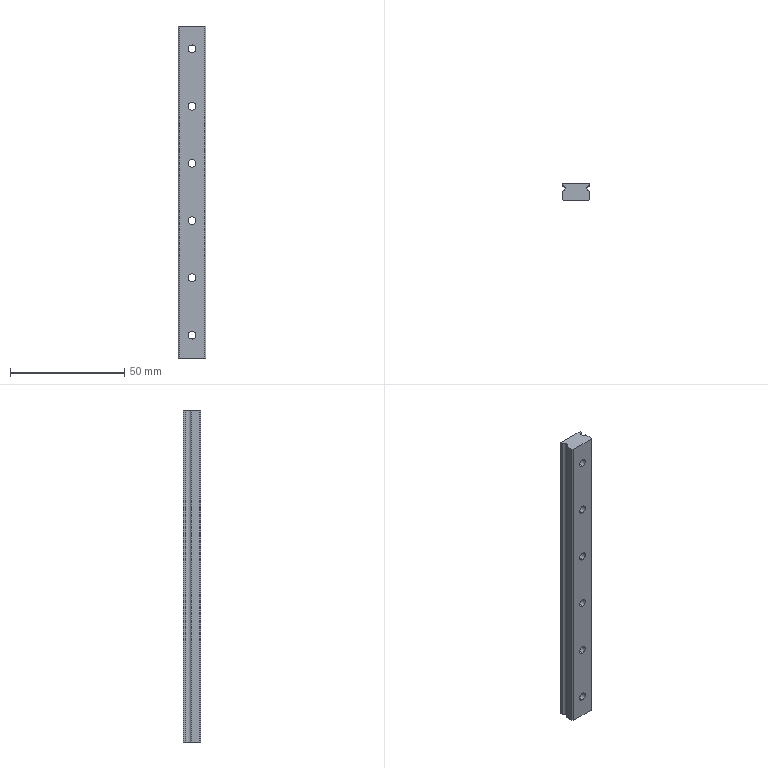Part | NX | features BREP 1 | 1 solid | 43 faces | box 12 x 7.5 x 145 mm | volume 11365 mm3 | cylinder 27 | plane 16 | commonest cylinder face diameters 3.5 x12 6 x12 2.5 x3
STEP:
#1=CARTESIAN_POINT('',(0.,7.5,13.));
#2=VERTEX_POINT('',#1);
#3=CARTESIAN_POINT('',(0.,7.5,7.));
#4=VERTEX_POINT('',#3);
#5=CARTESIAN_POINT('',(0.,7.5,10.));
#6=DIRECTION('',(0.,-1.,0.));
#7=DIRECTION('',(0.,0.,-1.));
#8=AXIS2_PLACEMENT_3D('',#5,#6,#7);
#9=CIRCLE('',#8,3.);
#10=EDGE_CURVE('',#2,#4,#9,.T.);
#11=ORIENTED_EDGE('',*,*,#10,.F.);
#12=CARTESIAN_POINT('',(0.,3.,13.));
#13=VERTEX_POINT('',#12);
#14=CARTESIAN_POINT('',(0.,5.25,13.));
#15=DIRECTION('',(0.,-1.,0.));
#16=VECTOR('',#15,1000.);
#17=LINE('',#14,#16);
#18=EDGE_CURVE('',#2,#13,#17,.T.);
#19=ORIENTED_EDGE('',*,*,#18,.T.);
#20=CARTESIAN_POINT('',(0.,3.,7.));
#21=VERTEX_POINT('',#20);
#22=CARTESIAN_POINT('',(0.,3.,10.));
#23=DIRECTION('',(0.,1.,0.));
#24=DIRECTION('',(0.,0.,-1.));
#25=AXIS2_PLACEMENT_3D('',#22,#23,#24);
#26=CIRCLE('',#25,3.);
#27=EDGE_CURVE('',#21,#13,#26,.T.);
#28=ORIENTED_EDGE('',*,*,#27,.F.);
#29=CARTESIAN_POINT('',(0.,5.25,7.));
#30=DIRECTION('',(0.,-1.,0.));
#31=VECTOR('',#30,1000.);
#32=LINE('',#29,#31);
#33=EDGE_CURVE('',#4,#21,#32,.T.);
#34=ORIENTED_EDGE('',*,*,#33,.F.);
#35=EDGE_LOOP('',(#11,#19,#28,#34));
#36=FACE_BOUND('',#35,.T.);
#37=CARTESIAN_POINT('',(0.,5.25,10.));
#38=DIRECTION('',(0.,-1.,0.));
#39=DIRECTION('',(0.,0.,-1.));
#40=AXIS2_PLACEMENT_3D('',#37,#38,#39);
#41=CYLINDRICAL_SURFACE('',#40,3.);
#42=ADVANCED_FACE('',(#36),#41,.F.);
#43=CARTESIAN_POINT('',(0.,7.5,138.));
#44=VERTEX_POINT('',#43);
#45=CARTESIAN_POINT('',(0.,7.5,132.));
#46=VERTEX_POINT('',#45);
#47=CARTESIAN_POINT('',(0.,7.5,135.));
#48=DIRECTION('',(0.,-1.,0.));
#49=DIRECTION('',(0.,0.,-1.));
#50=AXIS2_PLACEMENT_3D('',#47,#48,#49);
#51=CIRCLE('',#50,3.);
#52=EDGE_CURVE('',#44,#46,#51,.T.);
#53=ORIENTED_EDGE('',*,*,#52,.F.);
#54=CARTESIAN_POINT('',(0.,3.,138.));
#55=VERTEX_POINT('',#54);
#56=CARTESIAN_POINT('',(0.,5.25,138.));
#57=DIRECTION('',(0.,-1.,0.));
#58=VECTOR('',#57,1000.);
#59=LINE('',#56,#58);
#60=EDGE_CURVE('',#44,#55,#59,.T.);
#61=ORIENTED_EDGE('',*,*,#60,.T.);
#62=CARTESIAN_POINT('',(0.,3.,132.));
#63=VERTEX_POINT('',#62);
#64=CARTESIAN_POINT('',(0.,3.,135.));
#65=DIRECTION('',(0.,1.,0.));
#66=DIRECTION('',(0.,0.,-1.));
#67=AXIS2_PLACEMENT_3D('',#64,#65,#66);
#68=CIRCLE('',#67,3.);
#69=EDGE_CURVE('',#63,#55,#68,.T.);
#70=ORIENTED_EDGE('',*,*,#69,.F.);
#71=CARTESIAN_POINT('',(0.,5.25,132.));
#72=DIRECTION('',(0.,-1.,0.));
#73=VECTOR('',#72,1000.);
#74=LINE('',#71,#73);
#75=EDGE_CURVE('',#46,#63,#74,.T.);
#76=ORIENTED_EDGE('',*,*,#75,.F.);
#77=EDGE_LOOP('',(#53,#61,#70,#76));
#78=FACE_BOUND('',#77,.T.);
#79=CARTESIAN_POINT('',(0.,5.25,135.));
#80=DIRECTION('',(0.,-1.,0.));
#81=DIRECTION('',(0.,0.,-1.));
#82=AXIS2_PLACEMENT_3D('',#79,#80,#81);
#83=CYLINDRICAL_SURFACE('',#82,3.);
#84=ADVANCED_FACE('',(#78),#83,.F.);
#85=CARTESIAN_POINT('',(0.,7.5,113.));
#86=VERTEX_POINT('',#85);
#87=CARTESIAN_POINT('',(0.,7.5,107.));
#88=VERTEX_POINT('',#87);
#89=CARTESIAN_POINT('',(0.,7.5,110.));
#90=DIRECTION('',(0.,-1.,0.));
#91=DIRECTION('',(0.,0.,-1.));
#92=AXIS2_PLACEMENT_3D('',#89,#90,#91);
#93=CIRCLE('',#92,3.);
#94=EDGE_CURVE('',#86,#88,#93,.T.);
#95=ORIENTED_EDGE('',*,*,#94,.F.);
#96=CARTESIAN_POINT('',(0.,3.,113.));
#97=VERTEX_POINT('',#96);
#98=CARTESIAN_POINT('',(0.,5.25,113.));
#99=DIRECTION('',(0.,-1.,0.));
#100=VECTOR('',#99,1000.);
#101=LINE('',#98,#100);
#102=EDGE_CURVE('',#86,#97,#101,.T.);
#103=ORIENTED_EDGE('',*,*,#102,.T.);
#104=CARTESIAN_POINT('',(0.,3.,107.));
#105=VERTEX_POINT('',#104);
#106=CARTESIAN_POINT('',(0.,3.,110.));
#107=DIRECTION('',(0.,1.,0.));
#108=DIRECTION('',(0.,0.,-1.));
#109=AXIS2_PLACEMENT_3D('',#106,#107,#108);
#110=CIRCLE('',#109,3.);
#111=EDGE_CURVE('',#105,#97,#110,.T.);
#112=ORIENTED_EDGE('',*,*,#111,.F.);
#113=CARTESIAN_POINT('',(0.,5.25,107.));
#114=DIRECTION('',(0.,-1.,0.));
#115=VECTOR('',#114,1000.);
#116=LINE('',#113,#115);
#117=EDGE_CURVE('',#88,#105,#116,.T.);
#118=ORIENTED_EDGE('',*,*,#117,.F.);
#119=EDGE_LOOP('',(#95,#103,#112,#118));
#120=FACE_BOUND('',#119,.T.);
#121=CARTESIAN_POINT('',(0.,5.25,110.));
#122=DIRECTION('',(0.,-1.,0.));
#123=DIRECTION('',(0.,0.,-1.));
#124=AXIS2_PLACEMENT_3D('',#121,#122,#123);
#125=CYLINDRICAL_SURFACE('',#124,3.);
#126=ADVANCED_FACE('',(#120),#125,.F.);
#127=CARTESIAN_POINT('',(0.,7.5,88.));
#128=VERTEX_POINT('',#127);
#129=CARTESIAN_POINT('',(0.,7.5,82.));
#130=VERTEX_POINT('',#129);
#131=CARTESIAN_POINT('',(0.,7.5,85.));
#132=DIRECTION('',(0.,-1.,0.));
#133=DIRECTION('',(0.,0.,-1.));
#134=AXIS2_PLACEMENT_3D('',#131,#132,#133);
#135=CIRCLE('',#134,3.);
#136=EDGE_CURVE('',#128,#130,#135,.T.);
#137=ORIENTED_EDGE('',*,*,#136,.F.);
#138=CARTESIAN_POINT('',(0.,3.,88.));
#139=VERTEX_POINT('',#138);
#140=CARTESIAN_POINT('',(0.,5.25,88.));
#141=DIRECTION('',(0.,-1.,0.));
#142=VECTOR('',#141,1000.);
#143=LINE('',#140,#142);
#144=EDGE_CURVE('',#128,#139,#143,.T.);
#145=ORIENTED_EDGE('',*,*,#144,.T.);
#146=CARTESIAN_POINT('',(0.,3.,82.));
#147=VERTEX_POINT('',#146);
#148=CARTESIAN_POINT('',(0.,3.,85.));
#149=DIRECTION('',(0.,1.,0.));
#150=DIRECTION('',(0.,0.,-1.));
#151=AXIS2_PLACEMENT_3D('',#148,#149,#150);
#152=CIRCLE('',#151,3.);
#153=EDGE_CURVE('',#147,#139,#152,.T.);
#154=ORIENTED_EDGE('',*,*,#153,.F.);
#155=CARTESIAN_POINT('',(0.,5.25,82.));
#156=DIRECTION('',(0.,-1.,0.));
#157=VECTOR('',#156,1000.);
#158=LINE('',#155,#157);
#159=EDGE_CURVE('',#130,#147,#158,.T.);
#160=ORIENTED_EDGE('',*,*,#159,.F.);
#161=EDGE_LOOP('',(#137,#145,#154,#160));
#162=FACE_BOUND('',#161,.T.);
#163=CARTESIAN_POINT('',(0.,5.25,85.));
#164=DIRECTION('',(0.,-1.,0.));
#165=DIRECTION('',(0.,0.,-1.));
#166=AXIS2_PLACEMENT_3D('',#163,#164,#165);
#167=CYLINDRICAL_SURFACE('',#166,3.);
#168=ADVANCED_FACE('',(#162),#167,.F.);
#169=CARTESIAN_POINT('',(0.,7.5,63.));
#170=VERTEX_POINT('',#169);
#171=CARTESIAN_POINT('',(0.,7.5,57.));
#172=VERTEX_POINT('',#171);
#173=CARTESIAN_POINT('',(0.,7.5,60.));
#174=DIRECTION('',(0.,-1.,0.));
#175=DIRECTION('',(0.,0.,-1.));
#176=AXIS2_PLACEMENT_3D('',#173,#174,#175);
#177=CIRCLE('',#176,3.);
#178=EDGE_CURVE('',#170,#172,#177,.T.);
#179=ORIENTED_EDGE('',*,*,#178,.F.);
#180=CARTESIAN_POINT('',(0.,3.,63.));
#181=VERTEX_POINT('',#180);
#182=CARTESIAN_POINT('',(0.,5.25,63.));
#183=DIRECTION('',(0.,-1.,0.));
#184=VECTOR('',#183,1000.);
#185=LINE('',#182,#184);
#186=EDGE_CURVE('',#170,#181,#185,.T.);
#187=ORIENTED_EDGE('',*,*,#186,.T.);
#188=CARTESIAN_POINT('',(0.,3.,57.));
#189=VERTEX_POINT('',#188);
#190=CARTESIAN_POINT('',(0.,3.,60.));
#191=DIRECTION('',(0.,1.,0.));
#192=DIRECTION('',(0.,0.,-1.));
#193=AXIS2_PLACEMENT_3D('',#190,#191,#192);
#194=CIRCLE('',#193,3.);
#195=EDGE_CURVE('',#189,#181,#194,.T.);
#196=ORIENTED_EDGE('',*,*,#195,.F.);
#197=CARTESIAN_POINT('',(0.,5.25,57.));
#198=DIRECTION('',(0.,-1.,0.));
#199=VECTOR('',#198,1000.);
#200=LINE('',#197,#199);
#201=EDGE_CURVE('',#172,#189,#200,.T.);
#202=ORIENTED_EDGE('',*,*,#201,.F.);
#203=EDGE_LOOP('',(#179,#187,#196,#202));
#204=FACE_BOUND('',#203,.T.);
#205=CARTESIAN_POINT('',(0.,5.25,60.));
#206=DIRECTION('',(0.,-1.,0.));
#207=DIRECTION('',(0.,0.,-1.));
#208=AXIS2_PLACEMENT_3D('',#205,#206,#207);
#209=CYLINDRICAL_SURFACE('',#208,3.);
#210=ADVANCED_FACE('',(#204),#209,.F.);
#211=CARTESIAN_POINT('',(0.,7.5,38.));
#212=VERTEX_POINT('',#211);
#213=CARTESIAN_POINT('',(0.,7.5,32.));
#214=VERTEX_POINT('',#213);
#215=CARTESIAN_POINT('',(0.,7.5,35.));
#216=DIRECTION('',(0.,-1.,0.));
#217=DIRECTION('',(0.,0.,-1.));
#218=AXIS2_PLACEMENT_3D('',#215,#216,#217);
#219=CIRCLE('',#218,3.);
#220=EDGE_CURVE('',#212,#214,#219,.T.);
#221=ORIENTED_EDGE('',*,*,#220,.F.);
#222=CARTESIAN_POINT('',(0.,3.,38.));
#223=VERTEX_POINT('',#222);
#224=CARTESIAN_POINT('',(0.,5.25,38.));
#225=DIRECTION('',(0.,-1.,0.));
#226=VECTOR('',#225,1000.);
#227=LINE('',#224,#226);
#228=EDGE_CURVE('',#212,#223,#227,.T.);
#229=ORIENTED_EDGE('',*,*,#228,.T.);
#230=CARTESIAN_POINT('',(0.,3.,32.));
#231=VERTEX_POINT('',#230);
#232=CARTESIAN_POINT('',(0.,3.,35.));
#233=DIRECTION('',(0.,1.,0.));
#234=DIRECTION('',(0.,0.,-1.));
#235=AXIS2_PLACEMENT_3D('',#232,#233,#234);
#236=CIRCLE('',#235,3.);
#237=EDGE_CURVE('',#231,#223,#236,.T.);
#238=ORIENTED_EDGE('',*,*,#237,.F.);
#239=CARTESIAN_POINT('',(0.,5.25,32.));
#240=DIRECTION('',(0.,-1.,0.));
#241=VECTOR('',#240,1000.);
#242=LINE('',#239,#241);
#243=EDGE_CURVE('',#214,#231,#242,.T.);
#244=ORIENTED_EDGE('',*,*,#243,.F.);
#245=EDGE_LOOP('',(#221,#229,#238,#244));
#246=FACE_BOUND('',#245,.T.);
#247=CARTESIAN_POINT('',(0.,5.25,35.));
#248=DIRECTION('',(0.,-1.,0.));
#249=DIRECTION('',(0.,0.,-1.));
#250=AXIS2_PLACEMENT_3D('',#247,#248,#249);
#251=CYLINDRICAL_SURFACE('',#250,3.);
#252=ADVANCED_FACE('',(#246),#251,.F.);
#253=CARTESIAN_POINT('',(4.75,5.25,145.));
#254=VERTEX_POINT('',#253);
#255=CARTESIAN_POINT('',(6.,6.5,145.));
#256=VERTEX_POINT('',#255);
#257=CARTESIAN_POINT('',(6.,5.25,145.));
#258=DIRECTION('',(0.,0.,-1.));
#259=DIRECTION('',(-1.,0.,0.));
#260=AXIS2_PLACEMENT_3D('',#257,#258,#259);
#261=CIRCLE('',#260,1.25);
#262=EDGE_CURVE('',#254,#256,#261,.T.);
#263=ORIENTED_EDGE('',*,*,#262,.F.);
#264=CARTESIAN_POINT('',(4.75,5.25,0.));
#265=VERTEX_POINT('',#264);
#266=CARTESIAN_POINT('',(4.75,5.25,0.));
#267=DIRECTION('',(0.,0.,-1.));
#268=VECTOR('',#267,1000.);
#269=LINE('',#266,#268);
#270=EDGE_CURVE('',#254,#265,#269,.T.);
#271=ORIENTED_EDGE('',*,*,#270,.T.);
#272=CARTESIAN_POINT('',(6.,6.5,0.));
#273=VERTEX_POINT('',#272);
#274=CARTESIAN_POINT('',(6.,5.25,0.));
#275=DIRECTION('',(0.,0.,-1.));
#276=DIRECTION('',(-1.,0.,0.));
#277=AXIS2_PLACEMENT_3D('',#274,#275,#276);
#278=CIRCLE('',#277,1.25);
#279=EDGE_CURVE('',#265,#273,#278,.T.);
#280=ORIENTED_EDGE('',*,*,#279,.T.);
#281=CARTESIAN_POINT('',(6.,6.5,0.));
#282=DIRECTION('',(0.,0.,-1.));
#283=VECTOR('',#282,1000.);
#284=LINE('',#281,#283);
#285=EDGE_CURVE('',#256,#273,#284,.T.);
#286=ORIENTED_EDGE('',*,*,#285,.F.);
#287=EDGE_LOOP('',(#263,#271,#280,#286));
#288=FACE_BOUND('',#287,.T.);
#289=CARTESIAN_POINT('',(6.,5.25,0.));
#290=DIRECTION('',(0.,0.,-1.));
#291=DIRECTION('',(-1.,0.,0.));
#292=AXIS2_PLACEMENT_3D('',#289,#290,#291);
#293=CYLINDRICAL_SURFACE('',#292,1.25);
#294=ADVANCED_FACE('',(#288),#293,.F.);
#295=CARTESIAN_POINT('',(0.,3.,8.25));
#296=VERTEX_POINT('',#295);
#297=CARTESIAN_POINT('',(0.,3.,11.75));
#298=VERTEX_POINT('',#297);
#299=CARTESIAN_POINT('',(0.,3.,10.));
#300=DIRECTION('',(0.,1.,0.));
#301=DIRECTION('',(0.,0.,-1.));
#302=AXIS2_PLACEMENT_3D('',#299,#300,#301);
#303=CIRCLE('',#302,1.75);
#304=EDGE_CURVE('',#296,#298,#303,.T.);
#305=ORIENTED_EDGE('',*,*,#304,.T.);
#306=CARTESIAN_POINT('',(0.,0.,11.75));
#307=VERTEX_POINT('',#306);
#308=CARTESIAN_POINT('',(0.,1.5,11.75));
#309=DIRECTION('',(0.,-1.,0.));
#310=VECTOR('',#309,1000.);
#311=LINE('',#308,#310);
#312=EDGE_CURVE('',#298,#307,#311,.T.);
#313=ORIENTED_EDGE('',*,*,#312,.T.);
#314=CARTESIAN_POINT('',(0.,0.,8.25));
#315=VERTEX_POINT('',#314);
#316=CARTESIAN_POINT('',(0.,0.,10.));
#317=DIRECTION('',(0.,1.,0.));
#318=DIRECTION('',(0.,0.,-1.));
#319=AXIS2_PLACEMENT_3D('',#316,#317,#318);
#320=CIRCLE('',#319,1.75);
#321=EDGE_CURVE('',#315,#307,#320,.T.);
#322=ORIENTED_EDGE('',*,*,#321,.F.);
#323=CARTESIAN_POINT('',(0.,1.5,8.25));
#324=DIRECTION('',(0.,-1.,0.));
#325=VECTOR('',#324,1000.);
#326=LINE('',#323,#325);
#327=EDGE_CURVE('',#296,#315,#326,.T.);
#328=ORIENTED_EDGE('',*,*,#327,.F.);
#329=EDGE_LOOP('',(#305,#313,#322,#328));
#330=FACE_BOUND('',#329,.T.);
#331=CARTESIAN_POINT('',(0.,1.5,10.));
#332=DIRECTION('',(0.,-1.,0.));
#333=DIRECTION('',(0.,0.,-1.));
#334=AXIS2_PLACEMENT_3D('',#331,#332,#333);
#335=CYLINDRICAL_SURFACE('',#334,1.75);
#336=ADVANCED_FACE('',(#330),#335,.F.);
#337=CARTESIAN_POINT('',(0.,3.,133.25));
#338=VERTEX_POINT('',#337);
#339=CARTESIAN_POINT('',(0.,3.,136.75));
#340=VERTEX_POINT('',#339);
#341=CARTESIAN_POINT('',(0.,3.,135.));
#342=DIRECTION('',(0.,1.,0.));
#343=DIRECTION('',(0.,0.,-1.));
#344=AXIS2_PLACEMENT_3D('',#341,#342,#343);
#345=CIRCLE('',#344,1.75);
#346=EDGE_CURVE('',#338,#340,#345,.T.);
#347=ORIENTED_EDGE('',*,*,#346,.T.);
#348=CARTESIAN_POINT('',(0.,0.,136.75));
#349=VERTEX_POINT('',#348);
#350=CARTESIAN_POINT('',(0.,1.5,136.75));
#351=DIRECTION('',(0.,-1.,0.));
#352=VECTOR('',#351,1000.);
#353=LINE('',#350,#352);
#354=EDGE_CURVE('',#340,#349,#353,.T.);
#355=ORIENTED_EDGE('',*,*,#354,.T.);
#356=CARTESIAN_POINT('',(0.,0.,133.25));
#357=VERTEX_POINT('',#356);
#358=CARTESIAN_POINT('',(0.,0.,135.));
#359=DIRECTION('',(0.,1.,0.));
#360=DIRECTION('',(0.,0.,-1.));
#361=AXIS2_PLACEMENT_3D('',#358,#359,#360);
#362=CIRCLE('',#361,1.75);
#363=EDGE_CURVE('',#357,#349,#362,.T.);
#364=ORIENTED_EDGE('',*,*,#363,.F.);
#365=CARTESIAN_POINT('',(0.,1.5,133.25));
#366=DIRECTION('',(0.,-1.,0.));
#367=VECTOR('',#366,1000.);
#368=LINE('',#365,#367);
#369=EDGE_CURVE('',#338,#357,#368,.T.);
#370=ORIENTED_EDGE('',*,*,#369,.F.);
#371=EDGE_LOOP('',(#347,#355,#364,#370));
#372=FACE_BOUND('',#371,.T.);
#373=CARTESIAN_POINT('',(0.,1.5,135.));
#374=DIRECTION('',(0.,-1.,0.));
#375=DIRECTION('',(0.,0.,-1.));
#376=AXIS2_PLACEMENT_3D('',#373,#374,#375);
#377=CYLINDRICAL_SURFACE('',#376,1.75);
#378=ADVANCED_FACE('',(#372),#377,.F.);
#379=CARTESIAN_POINT('',(0.,3.,108.25));
#380=VERTEX_POINT('',#379);
#381=CARTESIAN_POINT('',(0.,3.,111.75));
#382=VERTEX_POINT('',#381);
#383=CARTESIAN_POINT('',(0.,3.,110.));
#384=DIRECTION('',(0.,1.,0.));
#385=DIRECTION('',(0.,0.,-1.));
#386=AXIS2_PLACEMENT_3D('',#383,#384,#385);
#387=CIRCLE('',#386,1.75);
#388=EDGE_CURVE('',#380,#382,#387,.T.);
#389=ORIENTED_EDGE('',*,*,#388,.T.);
#390=CARTESIAN_POINT('',(0.,0.,111.75));
#391=VERTEX_POINT('',#390);
#392=CARTESIAN_POINT('',(0.,1.5,111.75));
#393=DIRECTION('',(0.,-1.,0.));
#394=VECTOR('',#393,1000.);
#395=LINE('',#392,#394);
#396=EDGE_CURVE('',#382,#391,#395,.T.);
#397=ORIENTED_EDGE('',*,*,#396,.T.);
#398=CARTESIAN_POINT('',(0.,0.,108.25));
#399=VERTEX_POINT('',#398);
#400=CARTESIAN_POINT('',(0.,0.,110.));
#401=DIRECTION('',(0.,1.,0.));
#402=DIRECTION('',(0.,0.,-1.));
#403=AXIS2_PLACEMENT_3D('',#400,#401,#402);
#404=CIRCLE('',#403,1.75);
#405=EDGE_CURVE('',#399,#391,#404,.T.);
#406=ORIENTED_EDGE('',*,*,#405,.F.);
#407=CARTESIAN_POINT('',(0.,1.5,108.25));
#408=DIRECTION('',(0.,-1.,0.));
#409=VECTOR('',#408,1000.);
#410=LINE('',#407,#409);
#411=EDGE_CURVE('',#380,#399,#410,.T.);
#412=ORIENTED_EDGE('',*,*,#411,.F.);
#413=EDGE_LOOP('',(#389,#397,#406,#412));
#414=FACE_BOUND('',#413,.T.);
#415=CARTESIAN_POINT('',(0.,1.5,110.));
#416=DIRECTION('',(0.,-1.,0.));
#417=DIRECTION('',(0.,0.,-1.));
#418=AXIS2_PLACEMENT_3D('',#415,#416,#417);
#419=CYLINDRICAL_SURFACE('',#418,1.75);
#420=ADVANCED_FACE('',(#414),#419,.F.);
#421=CARTESIAN_POINT('',(0.,3.,83.25));
#422=VERTEX_POINT('',#421);
#423=CARTESIAN_POINT('',(0.,3.,86.75));
#424=VERTEX_POINT('',#423);
#425=CARTESIAN_POINT('',(0.,3.,85.));
#426=DIRECTION('',(0.,1.,0.));
#427=DIRECTION('',(0.,0.,-1.));
#428=AXIS2_PLACEMENT_3D('',#425,#426,#427);
#429=CIRCLE('',#428,1.75);
#430=EDGE_CURVE('',#422,#424,#429,.T.);
#431=ORIENTED_EDGE('',*,*,#430,.T.);
#432=CARTESIAN_POINT('',(0.,0.,86.75));
#433=VERTEX_POINT('',#432);
#434=CARTESIAN_POINT('',(0.,1.5,86.75));
#435=DIRECTION('',(0.,-1.,0.));
#436=VECTOR('',#435,1000.);
#437=LINE('',#434,#436);
#438=EDGE_CURVE('',#424,#433,#437,.T.);
#439=ORIENTED_EDGE('',*,*,#438,.T.);
#440=CARTESIAN_POINT('',(0.,0.,83.25));
#441=VERTEX_POINT('',#440);
#442=CARTESIAN_POINT('',(0.,0.,85.));
#443=DIRECTION('',(0.,1.,0.));
#444=DIRECTION('',(0.,0.,-1.));
#445=AXIS2_PLACEMENT_3D('',#442,#443,#444);
#446=CIRCLE('',#445,1.75);
#447=EDGE_CURVE('',#441,#433,#446,.T.);
#448=ORIENTED_EDGE('',*,*,#447,.F.);
#449=CARTESIAN_POINT('',(0.,1.5,83.25));
#450=DIRECTION('',(0.,-1.,0.));
#451=VECTOR('',#450,1000.);
#452=LINE('',#449,#451);
#453=EDGE_CURVE('',#422,#441,#452,.T.);
#454=ORIENTED_EDGE('',*,*,#453,.F.);
#455=EDGE_LOOP('',(#431,#439,#448,#454));
#456=FACE_BOUND('',#455,.T.);
#457=CARTESIAN_POINT('',(0.,1.5,85.));
#458=DIRECTION('',(0.,-1.,0.));
#459=DIRECTION('',(0.,0.,-1.));
#460=AXIS2_PLACEMENT_3D('',#457,#458,#459);
#461=CYLINDRICAL_SURFACE('',#460,1.75);
#462=ADVANCED_FACE('',(#456),#461,.F.);
#463=CARTESIAN_POINT('',(0.,3.,58.25));
#464=VERTEX_POINT('',#463);
#465=CARTESIAN_POINT('',(0.,3.,61.75));
#466=VERTEX_POINT('',#465);
#467=CARTESIAN_POINT('',(0.,3.,60.));
#468=DIRECTION('',(0.,1.,0.));
#469=DIRECTION('',(0.,0.,-1.));
#470=AXIS2_PLACEMENT_3D('',#467,#468,#469);
#471=CIRCLE('',#470,1.75);
#472=EDGE_CURVE('',#464,#466,#471,.T.);
#473=ORIENTED_EDGE('',*,*,#472,.T.);
#474=CARTESIAN_POINT('',(0.,0.,61.75));
#475=VERTEX_POINT('',#474);
#476=CARTESIAN_POINT('',(0.,1.5,61.75));
#477=DIRECTION('',(0.,-1.,0.));
#478=VECTOR('',#477,1000.);
#479=LINE('',#476,#478);
#480=EDGE_CURVE('',#466,#475,#479,.T.);
#481=ORIENTED_EDGE('',*,*,#480,.T.);
#482=CARTESIAN_POINT('',(0.,0.,58.25));
#483=VERTEX_POINT('',#482);
#484=CARTESIAN_POINT('',(0.,0.,60.));
#485=DIRECTION('',(0.,1.,0.));
#486=DIRECTION('',(0.,0.,-1.));
#487=AXIS2_PLACEMENT_3D('',#484,#485,#486);
#488=CIRCLE('',#487,1.75);
#489=EDGE_CURVE('',#483,#475,#488,.T.);
#490=ORIENTED_EDGE('',*,*,#489,.F.);
#491=CARTESIAN_POINT('',(0.,1.5,58.25));
#492=DIRECTION('',(0.,-1.,0.));
#493=VECTOR('',#492,1000.);
#494=LINE('',#491,#493);
#495=EDGE_CURVE('',#464,#483,#494,.T.);
#496=ORIENTED_EDGE('',*,*,#495,.F.);
#497=EDGE_LOOP('',(#473,#481,#490,#496));
#498=FACE_BOUND('',#497,.T.);
#499=CARTESIAN_POINT('',(0.,1.5,60.));
#500=DIRECTION('',(0.,-1.,0.));
#501=DIRECTION('',(0.,0.,-1.));
#502=AXIS2_PLACEMENT_3D('',#499,#500,#501);
#503=CYLINDRICAL_SURFACE('',#502,1.75);
#504=ADVANCED_FACE('',(#498),#503,.F.);
#505=CARTESIAN_POINT('',(0.,3.,33.25));
#506=VERTEX_POINT('',#505);
#507=CARTESIAN_POINT('',(0.,3.,36.75));
#508=VERTEX_POINT('',#507);
#509=CARTESIAN_POINT('',(0.,3.,35.));
#510=DIRECTION('',(0.,1.,0.));
#511=DIRECTION('',(0.,0.,-1.));
#512=AXIS2_PLACEMENT_3D('',#509,#510,#511);
#513=CIRCLE('',#512,1.75);
#514=EDGE_CURVE('',#506,#508,#513,.T.);
#515=ORIENTED_EDGE('',*,*,#514,.T.);
#516=CARTESIAN_POINT('',(0.,0.,36.75));
#517=VERTEX_POINT('',#516);
#518=CARTESIAN_POINT('',(0.,1.5,36.75));
#519=DIRECTION('',(0.,-1.,0.));
#520=VECTOR('',#519,1000.);
#521=LINE('',#518,#520);
#522=EDGE_CURVE('',#508,#517,#521,.T.);
#523=ORIENTED_EDGE('',*,*,#522,.T.);
#524=CARTESIAN_POINT('',(0.,0.,33.25));
#525=VERTEX_POINT('',#524);
#526=CARTESIAN_POINT('',(0.,0.,35.));
#527=DIRECTION('',(0.,1.,0.));
#528=DIRECTION('',(0.,0.,-1.));
#529=AXIS2_PLACEMENT_3D('',#526,#527,#528);
#530=CIRCLE('',#529,1.75);
#531=EDGE_CURVE('',#525,#517,#530,.T.);
#532=ORIENTED_EDGE('',*,*,#531,.F.);
#533=CARTESIAN_POINT('',(0.,1.5,33.25));
#534=DIRECTION('',(0.,-1.,0.));
#535=VECTOR('',#534,1000.);
#536=LINE('',#533,#535);
#537=EDGE_CURVE('',#506,#525,#536,.T.);
#538=ORIENTED_EDGE('',*,*,#537,.F.);
#539=EDGE_LOOP('',(#515,#523,#532,#538));
#540=FACE_BOUND('',#539,.T.);
#541=CARTESIAN_POINT('',(0.,1.5,35.));
#542=DIRECTION('',(0.,-1.,0.));
#543=DIRECTION('',(0.,0.,-1.));
#544=AXIS2_PLACEMENT_3D('',#541,#542,#543);
#545=CYLINDRICAL_SURFACE('',#544,1.75);
#546=ADVANCED_FACE('',(#540),#545,.F.);
#547=CARTESIAN_POINT('',(6.,7.5,0.));
#548=VERTEX_POINT('',#547);
#549=CARTESIAN_POINT('',(-6.,7.5,0.));
#550=VERTEX_POINT('',#549);
#551=CARTESIAN_POINT('',(-6.,7.5,0.));
#552=DIRECTION('',(-1.,0.,0.));
#553=VECTOR('',#552,1000.);
#554=LINE('',#551,#553);
#555=EDGE_CURVE('',#548,#550,#554,.T.);
#556=ORIENTED_EDGE('',*,*,#555,.T.);
#557=CARTESIAN_POINT('',(-6.,7.5,145.));
#558=VERTEX_POINT('',#557);
#559=CARTESIAN_POINT('',(-6.,7.5,0.));
#560=DIRECTION('',(0.,0.,1.));
#561=VECTOR('',#560,1000.);
#562=LINE('',#559,#561);
#563=EDGE_CURVE('',#550,#558,#562,.T.);
#564=ORIENTED_EDGE('',*,*,#563,.T.);
#565=CARTESIAN_POINT('',(6.,7.5,145.));
#566=VERTEX_POINT('',#565);
#567=CARTESIAN_POINT('',(-6.,7.5,145.));
#568=DIRECTION('',(1.,0.,0.));
#569=VECTOR('',#568,1000.);
#570=LINE('',#567,#569);
#571=EDGE_CURVE('',#558,#566,#570,.T.);
#572=ORIENTED_EDGE('',*,*,#571,.T.);
#573=CARTESIAN_POINT('',(6.,7.5,0.));
#574=DIRECTION('',(0.,0.,-1.));
#575=VECTOR('',#574,1000.);
#576=LINE('',#573,#575);
#577=EDGE_CURVE('',#566,#548,#576,.T.);
#578=ORIENTED_EDGE('',*,*,#577,.T.);
#579=EDGE_LOOP('',(#556,#564,#572,#578));
#580=FACE_BOUND('',#579,.T.);
#581=CARTESIAN_POINT('',(0.,7.5,10.));
#582=DIRECTION('',(0.,-1.,0.));
#583=DIRECTION('',(0.,0.,-1.));
#584=AXIS2_PLACEMENT_3D('',#581,#582,#583);
#585=CIRCLE('',#584,3.);
#586=EDGE_CURVE('',#4,#2,#585,.T.);
#587=ORIENTED_EDGE('',*,*,#586,.T.);
#588=ORIENTED_EDGE('',*,*,#10,.T.);
#589=EDGE_LOOP('',(#587,#588));
#590=FACE_BOUND('',#589,.T.);
#591=CARTESIAN_POINT('',(0.,7.5,135.));
#592=DIRECTION('',(0.,-1.,0.));
#593=DIRECTION('',(0.,0.,-1.));
#594=AXIS2_PLACEMENT_3D('',#591,#592,#593);
#595=CIRCLE('',#594,3.);
#596=EDGE_CURVE('',#46,#44,#595,.T.);
#597=ORIENTED_EDGE('',*,*,#596,.T.);
#598=ORIENTED_EDGE('',*,*,#52,.T.);
#599=EDGE_LOOP('',(#597,#598));
#600=FACE_BOUND('',#599,.T.);
#601=CARTESIAN_POINT('',(0.,7.5,110.));
#602=DIRECTION('',(0.,-1.,0.));
#603=DIRECTION('',(0.,0.,-1.));
#604=AXIS2_PLACEMENT_3D('',#601,#602,#603);
#605=CIRCLE('',#604,3.);
#606=EDGE_CURVE('',#88,#86,#605,.T.);
#607=ORIENTED_EDGE('',*,*,#606,.T.);
#608=ORIENTED_EDGE('',*,*,#94,.T.);
#609=EDGE_LOOP('',(#607,#608));
#610=FACE_BOUND('',#609,.T.);
#611=CARTESIAN_POINT('',(0.,7.5,85.));
#612=DIRECTION('',(0.,-1.,0.));
#613=DIRECTION('',(0.,0.,-1.));
#614=AXIS2_PLACEMENT_3D('',#611,#612,#613);
#615=CIRCLE('',#614,3.);
#616=EDGE_CURVE('',#130,#128,#615,.T.);
#617=ORIENTED_EDGE('',*,*,#616,.T.);
#618=ORIENTED_EDGE('',*,*,#136,.T.);
#619=EDGE_LOOP('',(#617,#618));
#620=FACE_BOUND('',#619,.T.);
#621=CARTESIAN_POINT('',(0.,7.5,60.));
#622=DIRECTION('',(0.,-1.,0.));
#623=DIRECTION('',(0.,0.,-1.));
#624=AXIS2_PLACEMENT_3D('',#621,#622,#623);
#625=CIRCLE('',#624,3.);
#626=EDGE_CURVE('',#172,#170,#625,.T.);
#627=ORIENTED_EDGE('',*,*,#626,.T.);
#628=ORIENTED_EDGE('',*,*,#178,.T.);
#629=EDGE_LOOP('',(#627,#628));
#630=FACE_BOUND('',#629,.T.);
#631=CARTESIAN_POINT('',(0.,7.5,35.));
#632=DIRECTION('',(0.,-1.,0.));
#633=DIRECTION('',(0.,0.,-1.));
#634=AXIS2_PLACEMENT_3D('',#631,#632,#633);
#635=CIRCLE('',#634,3.);
#636=EDGE_CURVE('',#214,#212,#635,.T.);
#637=ORIENTED_EDGE('',*,*,#636,.T.);
#638=ORIENTED_EDGE('',*,*,#220,.T.);
#639=EDGE_LOOP('',(#637,#638));
#640=FACE_BOUND('',#639,.T.);
#641=CARTESIAN_POINT('',(-6.,7.5,0.));
#642=DIRECTION('',(0.,1.,0.));
#643=DIRECTION('',(1.,0.,0.));
#644=AXIS2_PLACEMENT_3D('',#641,#642,#643);
#645=PLANE('',#644);
#646=ADVANCED_FACE('',(#580,#590,#600,#610,#620,#630,#640),#645,.T.);
#647=CARTESIAN_POINT('',(-6.,6.5,0.));
#648=VERTEX_POINT('',#647);
#649=CARTESIAN_POINT('',(-6.,6.5,0.));
#650=DIRECTION('',(0.,-1.,0.));
#651=VECTOR('',#650,1000.);
#652=LINE('',#649,#651);
#653=EDGE_CURVE('',#550,#648,#652,.T.);
#654=ORIENTED_EDGE('',*,*,#653,.T.);
#655=CARTESIAN_POINT('',(-6.,6.5,145.));
#656=VERTEX_POINT('',#655);
#657=CARTESIAN_POINT('',(-6.,6.5,0.));
#658=DIRECTION('',(0.,0.,1.));
#659=VECTOR('',#658,1000.);
#660=LINE('',#657,#659);
#661=EDGE_CURVE('',#648,#656,#660,.T.);
#662=ORIENTED_EDGE('',*,*,#661,.T.);
#663=CARTESIAN_POINT('',(-6.,6.5,145.));
#664=DIRECTION('',(0.,1.,0.));
#665=VECTOR('',#664,1000.);
#666=LINE('',#663,#665);
#667=EDGE_CURVE('',#656,#558,#666,.T.);
#668=ORIENTED_EDGE('',*,*,#667,.T.);
#669=ORIENTED_EDGE('',*,*,#563,.F.);
#670=EDGE_LOOP('',(#654,#662,#668,#669));
#671=FACE_BOUND('',#670,.T.);
#672=CARTESIAN_POINT('',(-6.,6.5,0.));
#673=DIRECTION('',(-1.,0.,0.));
#674=DIRECTION('',(0.,0.,1.));
#675=AXIS2_PLACEMENT_3D('',#672,#673,#674);
#676=PLANE('',#675);
#677=ADVANCED_FACE('',(#671),#676,.T.);
#678=ORIENTED_EDGE('',*,*,#555,.F.);
#679=CARTESIAN_POINT('',(6.,0.,0.));
#680=DIRECTION('',(0.,1.,0.));
#681=VECTOR('',#680,1000.);
#682=LINE('',#679,#681);
#683=EDGE_CURVE('',#273,#548,#682,.T.);
#684=ORIENTED_EDGE('',*,*,#683,.F.);
#685=ORIENTED_EDGE('',*,*,#279,.F.);
#686=CARTESIAN_POINT('',(6.,4.,0.));
#687=VERTEX_POINT('',#686);
#688=CARTESIAN_POINT('',(6.,5.25,0.));
#689=DIRECTION('',(0.,0.,-1.));
#690=DIRECTION('',(-1.,0.,0.));
#691=AXIS2_PLACEMENT_3D('',#688,#689,#690);
#692=CIRCLE('',#691,1.25);
#693=EDGE_CURVE('',#687,#265,#692,.T.);
#694=ORIENTED_EDGE('',*,*,#693,.F.);
#695=CARTESIAN_POINT('',(6.,0.5,0.));
#696=VERTEX_POINT('',#695);
#697=CARTESIAN_POINT('',(6.,0.,0.));
#698=DIRECTION('',(0.,1.,0.));
#699=VECTOR('',#698,1000.);
#700=LINE('',#697,#699);
#701=EDGE_CURVE('',#696,#687,#700,.T.);
#702=ORIENTED_EDGE('',*,*,#701,.F.);
#703=CARTESIAN_POINT('',(5.5,0.,0.));
#704=VERTEX_POINT('',#703);
#705=CARTESIAN_POINT('',(6.,0.5,0.));
#706=DIRECTION('',(0.7071,0.7071,0.));
#707=VECTOR('',#706,1000.);
#708=LINE('',#705,#707);
#709=EDGE_CURVE('',#704,#696,#708,.T.);
#710=ORIENTED_EDGE('',*,*,#709,.F.);
#711=CARTESIAN_POINT('',(-5.5,0.,0.));
#712=VERTEX_POINT('',#711);
#713=CARTESIAN_POINT('',(0.,0.,0.));
#714=DIRECTION('',(1.,0.,0.));
#715=VECTOR('',#714,1000.);
#716=LINE('',#713,#715);
#717=EDGE_CURVE('',#712,#704,#716,.T.);
#718=ORIENTED_EDGE('',*,*,#717,.F.);
#719=CARTESIAN_POINT('',(-6.,0.5,0.));
#720=VERTEX_POINT('',#719);
#721=CARTESIAN_POINT('',(-5.5,0.,0.));
#722=DIRECTION('',(0.7071,-0.7071,0.));
#723=VECTOR('',#722,1000.);
#724=LINE('',#721,#723);
#725=EDGE_CURVE('',#720,#712,#724,.T.);
#726=ORIENTED_EDGE('',*,*,#725,.F.);
#727=CARTESIAN_POINT('',(-6.,4.,0.));
#728=VERTEX_POINT('',#727);
#729=CARTESIAN_POINT('',(-6.,0.,0.));
#730=DIRECTION('',(0.,-1.,0.));
#731=VECTOR('',#730,1000.);
#732=LINE('',#729,#731);
#733=EDGE_CURVE('',#728,#720,#732,.T.);
#734=ORIENTED_EDGE('',*,*,#733,.F.);
#735=CARTESIAN_POINT('',(-6.,5.25,0.));
#736=DIRECTION('',(0.,0.,-1.));
#737=DIRECTION('',(-1.,0.,0.));
#738=AXIS2_PLACEMENT_3D('',#735,#736,#737);
#739=CIRCLE('',#738,1.25);
#740=EDGE_CURVE('',#648,#728,#739,.T.);
#741=ORIENTED_EDGE('',*,*,#740,.F.);
#742=ORIENTED_EDGE('',*,*,#653,.F.);
#743=EDGE_LOOP('',(#678,#684,#685,#694,#702,#710,#718,#726,#734,#741,#742));
#744=FACE_BOUND('',#743,.T.);
#745=CARTESIAN_POINT('',(0.,0.,0.));
#746=DIRECTION('',(0.,0.,1.));
#747=DIRECTION('',(1.,0.,0.));
#748=AXIS2_PLACEMENT_3D('',#745,#746,#747);
#749=PLANE('',#748);
#750=ADVANCED_FACE('',(#744),#749,.F.);
#751=ORIENTED_EDGE('',*,*,#683,.T.);
#752=ORIENTED_EDGE('',*,*,#577,.F.);
#753=CARTESIAN_POINT('',(6.,7.5,145.));
#754=DIRECTION('',(0.,-1.,0.));
#755=VECTOR('',#754,1000.);
#756=LINE('',#753,#755);
#757=EDGE_CURVE('',#566,#256,#756,.T.);
#758=ORIENTED_EDGE('',*,*,#757,.T.);
#759=ORIENTED_EDGE('',*,*,#285,.T.);
#760=EDGE_LOOP('',(#751,#752,#758,#759));
#761=FACE_BOUND('',#760,.T.);
#762=CARTESIAN_POINT('',(6.,7.5,0.));
#763=DIRECTION('',(1.,0.,0.));
#764=DIRECTION('',(0.,1.,0.));
#765=AXIS2_PLACEMENT_3D('',#762,#763,#764);
#766=PLANE('',#765);
#767=ADVANCED_FACE('',(#761),#766,.T.);
#768=CARTESIAN_POINT('',(6.,4.,145.));
#769=VERTEX_POINT('',#768);
#770=CARTESIAN_POINT('',(6.,5.25,145.));
#771=DIRECTION('',(0.,0.,-1.));
#772=DIRECTION('',(-1.,0.,0.));
#773=AXIS2_PLACEMENT_3D('',#770,#771,#772);
#774=CIRCLE('',#773,1.25);
#775=EDGE_CURVE('',#769,#254,#774,.T.);
#776=ORIENTED_EDGE('',*,*,#775,.T.);
#777=ORIENTED_EDGE('',*,*,#262,.T.);
#778=ORIENTED_EDGE('',*,*,#757,.F.);
#779=ORIENTED_EDGE('',*,*,#571,.F.);
#780=ORIENTED_EDGE('',*,*,#667,.F.);
#781=CARTESIAN_POINT('',(-6.,4.,145.));
#782=VERTEX_POINT('',#781);
#783=CARTESIAN_POINT('',(-6.,5.25,145.));
#784=DIRECTION('',(0.,0.,-1.));
#785=DIRECTION('',(-1.,0.,0.));
#786=AXIS2_PLACEMENT_3D('',#783,#784,#785);
#787=CIRCLE('',#786,1.25);
#788=EDGE_CURVE('',#656,#782,#787,.T.);
#789=ORIENTED_EDGE('',*,*,#788,.T.);
#790=CARTESIAN_POINT('',(-6.,0.5,145.));
#791=VERTEX_POINT('',#790);
#792=CARTESIAN_POINT('',(-6.,0.,145.));
#793=DIRECTION('',(0.,-1.,0.));
#794=VECTOR('',#793,1000.);
#795=LINE('',#792,#794);
#796=EDGE_CURVE('',#782,#791,#795,.T.);
#797=ORIENTED_EDGE('',*,*,#796,.T.);
#798=CARTESIAN_POINT('',(-5.5,0.,145.));
#799=VERTEX_POINT('',#798);
#800=CARTESIAN_POINT('',(-5.5,0.,145.));
#801=DIRECTION('',(-0.7071,0.7071,0.));
#802=VECTOR('',#801,1000.);
#803=LINE('',#800,#802);
#804=EDGE_CURVE('',#799,#791,#803,.T.);
#805=ORIENTED_EDGE('',*,*,#804,.F.);
#806=CARTESIAN_POINT('',(5.5,0.,145.));
#807=VERTEX_POINT('',#806);
#808=CARTESIAN_POINT('',(0.,0.,145.));
#809=DIRECTION('',(1.,0.,0.));
#810=VECTOR('',#809,1000.);
#811=LINE('',#808,#810);
#812=EDGE_CURVE('',#799,#807,#811,.T.);
#813=ORIENTED_EDGE('',*,*,#812,.T.);
#814=CARTESIAN_POINT('',(6.,0.5,145.));
#815=VERTEX_POINT('',#814);
#816=CARTESIAN_POINT('',(6.,0.5,145.));
#817=DIRECTION('',(-0.7071,-0.7071,0.));
#818=VECTOR('',#817,1000.);
#819=LINE('',#816,#818);
#820=EDGE_CURVE('',#815,#807,#819,.T.);
#821=ORIENTED_EDGE('',*,*,#820,.F.);
#822=CARTESIAN_POINT('',(6.,0.,145.));
#823=DIRECTION('',(0.,1.,0.));
#824=VECTOR('',#823,1000.);
#825=LINE('',#822,#824);
#826=EDGE_CURVE('',#815,#769,#825,.T.);
#827=ORIENTED_EDGE('',*,*,#826,.T.);
#828=EDGE_LOOP('',(#776,#777,#778,#779,#780,#789,#797,#805,#813,#821,#827));
#829=FACE_BOUND('',#828,.T.);
#830=CARTESIAN_POINT('',(0.,0.,145.));
#831=DIRECTION('',(0.,0.,1.));
#832=DIRECTION('',(1.,0.,0.));
#833=AXIS2_PLACEMENT_3D('',#830,#831,#832);
#834=PLANE('',#833);
#835=ADVANCED_FACE('',(#829),#834,.T.);
#836=ORIENTED_EDGE('',*,*,#18,.F.);
#837=ORIENTED_EDGE('',*,*,#586,.F.);
#838=ORIENTED_EDGE('',*,*,#33,.T.);
#839=CARTESIAN_POINT('',(0.,3.,10.));
#840=DIRECTION('',(0.,1.,0.));
#841=DIRECTION('',(0.,0.,-1.));
#842=AXIS2_PLACEMENT_3D('',#839,#840,#841);
#843=CIRCLE('',#842,3.);
#844=EDGE_CURVE('',#13,#21,#843,.T.);
#845=ORIENTED_EDGE('',*,*,#844,.F.);
#846=EDGE_LOOP('',(#836,#837,#838,#845));
#847=FACE_BOUND('',#846,.T.);
#848=CARTESIAN_POINT('',(0.,5.25,10.));
#849=DIRECTION('',(0.,-1.,0.));
#850=DIRECTION('',(0.,0.,-1.));
#851=AXIS2_PLACEMENT_3D('',#848,#849,#850);
#852=CYLINDRICAL_SURFACE('',#851,3.);
#853=ADVANCED_FACE('',(#847),#852,.F.);
#854=ORIENTED_EDGE('',*,*,#60,.F.);
#855=ORIENTED_EDGE('',*,*,#596,.F.);
#856=ORIENTED_EDGE('',*,*,#75,.T.);
#857=CARTESIAN_POINT('',(0.,3.,135.));
#858=DIRECTION('',(0.,1.,0.));
#859=DIRECTION('',(0.,0.,-1.));
#860=AXIS2_PLACEMENT_3D('',#857,#858,#859);
#861=CIRCLE('',#860,3.);
#862=EDGE_CURVE('',#55,#63,#861,.T.);
#863=ORIENTED_EDGE('',*,*,#862,.F.);
#864=EDGE_LOOP('',(#854,#855,#856,#863));
#865=FACE_BOUND('',#864,.T.);
#866=CARTESIAN_POINT('',(0.,5.25,135.));
#867=DIRECTION('',(0.,-1.,0.));
#868=DIRECTION('',(0.,0.,-1.));
#869=AXIS2_PLACEMENT_3D('',#866,#867,#868);
#870=CYLINDRICAL_SURFACE('',#869,3.);
#871=ADVANCED_FACE('',(#865),#870,.F.);
#872=ORIENTED_EDGE('',*,*,#102,.F.);
#873=ORIENTED_EDGE('',*,*,#606,.F.);
#874=ORIENTED_EDGE('',*,*,#117,.T.);
#875=CARTESIAN_POINT('',(0.,3.,110.));
#876=DIRECTION('',(0.,1.,0.));
#877=DIRECTION('',(0.,0.,-1.));
#878=AXIS2_PLACEMENT_3D('',#875,#876,#877);
#879=CIRCLE('',#878,3.);
#880=EDGE_CURVE('',#97,#105,#879,.T.);
#881=ORIENTED_EDGE('',*,*,#880,.F.);
#882=EDGE_LOOP('',(#872,#873,#874,#881));
#883=FACE_BOUND('',#882,.T.);
#884=CARTESIAN_POINT('',(0.,5.25,110.));
#885=DIRECTION('',(0.,-1.,0.));
#886=DIRECTION('',(0.,0.,-1.));
#887=AXIS2_PLACEMENT_3D('',#884,#885,#886);
#888=CYLINDRICAL_SURFACE('',#887,3.);
#889=ADVANCED_FACE('',(#883),#888,.F.);
#890=ORIENTED_EDGE('',*,*,#144,.F.);
#891=ORIENTED_EDGE('',*,*,#616,.F.);
#892=ORIENTED_EDGE('',*,*,#159,.T.);
#893=CARTESIAN_POINT('',(0.,3.,85.));
#894=DIRECTION('',(0.,1.,0.));
#895=DIRECTION('',(0.,0.,-1.));
#896=AXIS2_PLACEMENT_3D('',#893,#894,#895);
#897=CIRCLE('',#896,3.);
#898=EDGE_CURVE('',#139,#147,#897,.T.);
#899=ORIENTED_EDGE('',*,*,#898,.F.);
#900=EDGE_LOOP('',(#890,#891,#892,#899));
#901=FACE_BOUND('',#900,.T.);
#902=CARTESIAN_POINT('',(0.,5.25,85.));
#903=DIRECTION('',(0.,-1.,0.));
#904=DIRECTION('',(0.,0.,-1.));
#905=AXIS2_PLACEMENT_3D('',#902,#903,#904);
#906=CYLINDRICAL_SURFACE('',#905,3.);
#907=ADVANCED_FACE('',(#901),#906,.F.);
#908=ORIENTED_EDGE('',*,*,#186,.F.);
#909=ORIENTED_EDGE('',*,*,#626,.F.);
#910=ORIENTED_EDGE('',*,*,#201,.T.);
#911=CARTESIAN_POINT('',(0.,3.,60.));
#912=DIRECTION('',(0.,1.,0.));
#913=DIRECTION('',(0.,0.,-1.));
#914=AXIS2_PLACEMENT_3D('',#911,#912,#913);
#915=CIRCLE('',#914,3.);
#916=EDGE_CURVE('',#181,#189,#915,.T.);
#917=ORIENTED_EDGE('',*,*,#916,.F.);
#918=EDGE_LOOP('',(#908,#909,#910,#917));
#919=FACE_BOUND('',#918,.T.);
#920=CARTESIAN_POINT('',(0.,5.25,60.));
#921=DIRECTION('',(0.,-1.,0.));
#922=DIRECTION('',(0.,0.,-1.));
#923=AXIS2_PLACEMENT_3D('',#920,#921,#922);
#924=CYLINDRICAL_SURFACE('',#923,3.);
#925=ADVANCED_FACE('',(#919),#924,.F.);
#926=ORIENTED_EDGE('',*,*,#228,.F.);
#927=ORIENTED_EDGE('',*,*,#636,.F.);
#928=ORIENTED_EDGE('',*,*,#243,.T.);
#929=CARTESIAN_POINT('',(0.,3.,35.));
#930=DIRECTION('',(0.,1.,0.));
#931=DIRECTION('',(0.,0.,-1.));
#932=AXIS2_PLACEMENT_3D('',#929,#930,#931);
#933=CIRCLE('',#932,3.);
#934=EDGE_CURVE('',#223,#231,#933,.T.);
#935=ORIENTED_EDGE('',*,*,#934,.F.);
#936=EDGE_LOOP('',(#926,#927,#928,#935));
#937=FACE_BOUND('',#936,.T.);
#938=CARTESIAN_POINT('',(0.,5.25,35.));
#939=DIRECTION('',(0.,-1.,0.));
#940=DIRECTION('',(0.,0.,-1.));
#941=AXIS2_PLACEMENT_3D('',#938,#939,#940);
#942=CYLINDRICAL_SURFACE('',#941,3.);
#943=ADVANCED_FACE('',(#937),#942,.F.);
#944=ORIENTED_EDGE('',*,*,#661,.F.);
#945=ORIENTED_EDGE('',*,*,#740,.T.);
#946=CARTESIAN_POINT('',(-6.,4.,0.));
#947=DIRECTION('',(0.,0.,-1.));
#948=VECTOR('',#947,1000.);
#949=LINE('',#946,#948);
#950=EDGE_CURVE('',#782,#728,#949,.T.);
#951=ORIENTED_EDGE('',*,*,#950,.F.);
#952=ORIENTED_EDGE('',*,*,#788,.F.);
#953=EDGE_LOOP('',(#944,#945,#951,#952));
#954=FACE_BOUND('',#953,.T.);
#955=CARTESIAN_POINT('',(-6.,5.25,0.));
#956=DIRECTION('',(0.,0.,-1.));
#957=DIRECTION('',(-1.,0.,0.));
#958=AXIS2_PLACEMENT_3D('',#955,#956,#957);
#959=CYLINDRICAL_SURFACE('',#958,1.25);
#960=ADVANCED_FACE('',(#954),#959,.F.);
#961=ORIENTED_EDGE('',*,*,#270,.F.);
#962=ORIENTED_EDGE('',*,*,#775,.F.);
#963=CARTESIAN_POINT('',(6.,4.,0.));
#964=DIRECTION('',(0.,0.,1.));
#965=VECTOR('',#964,1000.);
#966=LINE('',#963,#965);
#967=EDGE_CURVE('',#687,#769,#966,.T.);
#968=ORIENTED_EDGE('',*,*,#967,.F.);
#969=ORIENTED_EDGE('',*,*,#693,.T.);
#970=EDGE_LOOP('',(#961,#962,#968,#969));
#971=FACE_BOUND('',#970,.T.);
#972=CARTESIAN_POINT('',(6.,5.25,0.));
#973=DIRECTION('',(0.,0.,-1.));
#974=DIRECTION('',(-1.,0.,0.));
#975=AXIS2_PLACEMENT_3D('',#972,#973,#974);
#976=CYLINDRICAL_SURFACE('',#975,1.25);
#977=ADVANCED_FACE('',(#971),#976,.F.);
#978=ORIENTED_EDGE('',*,*,#701,.T.);
#979=ORIENTED_EDGE('',*,*,#967,.T.);
#980=ORIENTED_EDGE('',*,*,#826,.F.);
#981=CARTESIAN_POINT('',(6.,0.5,0.));
#982=DIRECTION('',(0.,0.,-1.));
#983=VECTOR('',#982,1000.);
#984=LINE('',#981,#983);
#985=EDGE_CURVE('',#815,#696,#984,.T.);
#986=ORIENTED_EDGE('',*,*,#985,.T.);
#987=EDGE_LOOP('',(#978,#979,#980,#986));
#988=FACE_BOUND('',#987,.T.);
#989=CARTESIAN_POINT('',(6.,4.,0.));
#990=DIRECTION('',(1.,0.,0.));
#991=DIRECTION('',(0.,1.,0.));
#992=AXIS2_PLACEMENT_3D('',#989,#990,#991);
#993=PLANE('',#992);
#994=ADVANCED_FACE('',(#988),#993,.T.);
#995=ORIENTED_EDGE('',*,*,#717,.T.);
#996=CARTESIAN_POINT('',(5.5,0.,0.));
#997=DIRECTION('',(0.,0.,1.));
#998=VECTOR('',#997,1000.);
#999=LINE('',#996,#998);
#1000=EDGE_CURVE('',#704,#807,#999,.T.);
#1001=ORIENTED_EDGE('',*,*,#1000,.T.);
#1002=ORIENTED_EDGE('',*,*,#812,.F.);
#1003=CARTESIAN_POINT('',(-5.5,0.,0.));
#1004=DIRECTION('',(0.,0.,-1.));
#1005=VECTOR('',#1004,1000.);
#1006=LINE('',#1003,#1005);
#1007=EDGE_CURVE('',#799,#712,#1006,.T.);
#1008=ORIENTED_EDGE('',*,*,#1007,.T.);
#1009=EDGE_LOOP('',(#995,#1001,#1002,#1008));
#1010=FACE_BOUND('',#1009,.T.);
#1011=ORIENTED_EDGE('',*,*,#321,.T.);
#1012=CARTESIAN_POINT('',(0.,0.,10.));
#1013=DIRECTION('',(0.,1.,0.));
#1014=DIRECTION('',(0.,0.,-1.));
#1015=AXIS2_PLACEMENT_3D('',#1012,#1013,#1014);
#1016=CIRCLE('',#1015,1.75);
#1017=EDGE_CURVE('',#307,#315,#1016,.T.);
#1018=ORIENTED_EDGE('',*,*,#1017,.T.);
#1019=EDGE_LOOP('',(#1011,#1018));
#1020=FACE_BOUND('',#1019,.T.);
#1021=ORIENTED_EDGE('',*,*,#363,.T.);
#1022=CARTESIAN_POINT('',(0.,0.,135.));
#1023=DIRECTION('',(0.,1.,0.));
#1024=DIRECTION('',(0.,0.,-1.));
#1025=AXIS2_PLACEMENT_3D('',#1022,#1023,#1024);
#1026=CIRCLE('',#1025,1.75);
#1027=EDGE_CURVE('',#349,#357,#1026,.T.);
#1028=ORIENTED_EDGE('',*,*,#1027,.T.);
#1029=EDGE_LOOP('',(#1021,#1028));
#1030=FACE_BOUND('',#1029,.T.);
#1031=ORIENTED_EDGE('',*,*,#405,.T.);
#1032=CARTESIAN_POINT('',(0.,0.,110.));
#1033=DIRECTION('',(0.,1.,0.));
#1034=DIRECTION('',(0.,0.,-1.));
#1035=AXIS2_PLACEMENT_3D('',#1032,#1033,#1034);
#1036=CIRCLE('',#1035,1.75);
#1037=EDGE_CURVE('',#391,#399,#1036,.T.);
#1038=ORIENTED_EDGE('',*,*,#1037,.T.);
#1039=EDGE_LOOP('',(#1031,#1038));
#1040=FACE_BOUND('',#1039,.T.);
#1041=ORIENTED_EDGE('',*,*,#447,.T.);
#1042=CARTESIAN_POINT('',(0.,0.,85.));
#1043=DIRECTION('',(0.,1.,0.));
#1044=DIRECTION('',(0.,0.,-1.));
#1045=AXIS2_PLACEMENT_3D('',#1042,#1043,#1044);
#1046=CIRCLE('',#1045,1.75);
#1047=EDGE_CURVE('',#433,#441,#1046,.T.);
#1048=ORIENTED_EDGE('',*,*,#1047,.T.);
#1049=EDGE_LOOP('',(#1041,#1048));
#1050=FACE_BOUND('',#1049,.T.);
#1051=ORIENTED_EDGE('',*,*,#489,.T.);
#1052=CARTESIAN_POINT('',(0.,0.,60.));
#1053=DIRECTION('',(0.,1.,0.));
#1054=DIRECTION('',(0.,0.,-1.));
#1055=AXIS2_PLACEMENT_3D('',#1052,#1053,#1054);
#1056=CIRCLE('',#1055,1.75);
#1057=EDGE_CURVE('',#475,#483,#1056,.T.);
#1058=ORIENTED_EDGE('',*,*,#1057,.T.);
#1059=EDGE_LOOP('',(#1051,#1058));
#1060=FACE_BOUND('',#1059,.T.);
#1061=ORIENTED_EDGE('',*,*,#531,.T.);
#1062=CARTESIAN_POINT('',(0.,0.,35.));
#1063=DIRECTION('',(0.,1.,0.));
#1064=DIRECTION('',(0.,0.,-1.));
#1065=AXIS2_PLACEMENT_3D('',#1062,#1063,#1064);
#1066=CIRCLE('',#1065,1.75);
#1067=EDGE_CURVE('',#517,#525,#1066,.T.);
#1068=ORIENTED_EDGE('',*,*,#1067,.T.);
#1069=EDGE_LOOP('',(#1061,#1068));
#1070=FACE_BOUND('',#1069,.T.);
#1071=CARTESIAN_POINT('',(5.5,0.,0.));
#1072=DIRECTION('',(0.,-1.,0.));
#1073=DIRECTION('',(0.,0.,-1.));
#1074=AXIS2_PLACEMENT_3D('',#1071,#1072,#1073);
#1075=PLANE('',#1074);
#1076=ADVANCED_FACE('',(#1010,#1020,#1030,#1040,#1050,#1060,#1070),#1075,.T.);
#1077=ORIENTED_EDGE('',*,*,#733,.T.);
#1078=CARTESIAN_POINT('',(-6.,0.5,0.));
#1079=DIRECTION('',(0.,0.,1.));
#1080=VECTOR('',#1079,1000.);
#1081=LINE('',#1078,#1080);
#1082=EDGE_CURVE('',#720,#791,#1081,.T.);
#1083=ORIENTED_EDGE('',*,*,#1082,.T.);
#1084=ORIENTED_EDGE('',*,*,#796,.F.);
#1085=ORIENTED_EDGE('',*,*,#950,.T.);
#1086=EDGE_LOOP('',(#1077,#1083,#1084,#1085));
#1087=FACE_BOUND('',#1086,.T.);
#1088=CARTESIAN_POINT('',(-6.,0.5,0.));
#1089=DIRECTION('',(-1.,0.,0.));
#1090=DIRECTION('',(0.,0.,1.));
#1091=AXIS2_PLACEMENT_3D('',#1088,#1089,#1090);
#1092=PLANE('',#1091);
#1093=ADVANCED_FACE('',(#1087),#1092,.T.);
#1094=ORIENTED_EDGE('',*,*,#27,.T.);
#1095=ORIENTED_EDGE('',*,*,#844,.T.);
#1096=EDGE_LOOP('',(#1094,#1095));
#1097=FACE_BOUND('',#1096,.T.);
#1098=ORIENTED_EDGE('',*,*,#304,.F.);
#1099=CARTESIAN_POINT('',(0.,3.,10.));
#1100=DIRECTION('',(0.,1.,0.));
#1101=DIRECTION('',(0.,0.,-1.));
#1102=AXIS2_PLACEMENT_3D('',#1099,#1100,#1101);
#1103=CIRCLE('',#1102,1.75);
#1104=EDGE_CURVE('',#298,#296,#1103,.T.);
#1105=ORIENTED_EDGE('',*,*,#1104,.F.);
#1106=EDGE_LOOP('',(#1098,#1105));
#1107=FACE_BOUND('',#1106,.T.);
#1108=CARTESIAN_POINT('',(0.,3.,7.625));
#1109=DIRECTION('',(0.,-1.,0.));
#1110=DIRECTION('',(0.,0.,-1.));
#1111=AXIS2_PLACEMENT_3D('',#1108,#1109,#1110);
#1112=PLANE('',#1111);
#1113=ADVANCED_FACE('',(#1097,#1107),#1112,.F.);
#1114=ORIENTED_EDGE('',*,*,#69,.T.);
#1115=ORIENTED_EDGE('',*,*,#862,.T.);
#1116=EDGE_LOOP('',(#1114,#1115));
#1117=FACE_BOUND('',#1116,.T.);
#1118=ORIENTED_EDGE('',*,*,#346,.F.);
#1119=CARTESIAN_POINT('',(0.,3.,135.));
#1120=DIRECTION('',(0.,1.,0.));
#1121=DIRECTION('',(0.,0.,-1.));
#1122=AXIS2_PLACEMENT_3D('',#1119,#1120,#1121);
#1123=CIRCLE('',#1122,1.75);
#1124=EDGE_CURVE('',#340,#338,#1123,.T.);
#1125=ORIENTED_EDGE('',*,*,#1124,.F.);
#1126=EDGE_LOOP('',(#1118,#1125));
#1127=FACE_BOUND('',#1126,.T.);
#1128=CARTESIAN_POINT('',(0.,3.,132.625));
#1129=DIRECTION('',(0.,-1.,0.));
#1130=DIRECTION('',(0.,0.,-1.));
#1131=AXIS2_PLACEMENT_3D('',#1128,#1129,#1130);
#1132=PLANE('',#1131);
#1133=ADVANCED_FACE('',(#1117,#1127),#1132,.F.);
#1134=ORIENTED_EDGE('',*,*,#111,.T.);
#1135=ORIENTED_EDGE('',*,*,#880,.T.);
#1136=EDGE_LOOP('',(#1134,#1135));
#1137=FACE_BOUND('',#1136,.T.);
#1138=ORIENTED_EDGE('',*,*,#388,.F.);
#1139=CARTESIAN_POINT('',(0.,3.,110.));
#1140=DIRECTION('',(0.,1.,0.));
#1141=DIRECTION('',(0.,0.,-1.));
#1142=AXIS2_PLACEMENT_3D('',#1139,#1140,#1141);
#1143=CIRCLE('',#1142,1.75);
#1144=EDGE_CURVE('',#382,#380,#1143,.T.);
#1145=ORIENTED_EDGE('',*,*,#1144,.F.);
#1146=EDGE_LOOP('',(#1138,#1145));
#1147=FACE_BOUND('',#1146,.T.);
#1148=CARTESIAN_POINT('',(0.,3.,107.625));
#1149=DIRECTION('',(0.,-1.,0.));
#1150=DIRECTION('',(0.,0.,-1.));
#1151=AXIS2_PLACEMENT_3D('',#1148,#1149,#1150);
#1152=PLANE('',#1151);
#1153=ADVANCED_FACE('',(#1137,#1147),#1152,.F.);
#1154=ORIENTED_EDGE('',*,*,#153,.T.);
#1155=ORIENTED_EDGE('',*,*,#898,.T.);
#1156=EDGE_LOOP('',(#1154,#1155));
#1157=FACE_BOUND('',#1156,.T.);
#1158=ORIENTED_EDGE('',*,*,#430,.F.);
#1159=CARTESIAN_POINT('',(0.,3.,85.));
#1160=DIRECTION('',(0.,1.,0.));
#1161=DIRECTION('',(0.,0.,-1.));
#1162=AXIS2_PLACEMENT_3D('',#1159,#1160,#1161);
#1163=CIRCLE('',#1162,1.75);
#1164=EDGE_CURVE('',#424,#422,#1163,.T.);
#1165=ORIENTED_EDGE('',*,*,#1164,.F.);
#1166=EDGE_LOOP('',(#1158,#1165));
#1167=FACE_BOUND('',#1166,.T.);
#1168=CARTESIAN_POINT('',(0.,3.,82.625));
#1169=DIRECTION('',(0.,-1.,0.));
#1170=DIRECTION('',(0.,0.,-1.));
#1171=AXIS2_PLACEMENT_3D('',#1168,#1169,#1170);
#1172=PLANE('',#1171);
#1173=ADVANCED_FACE('',(#1157,#1167),#1172,.F.);
#1174=ORIENTED_EDGE('',*,*,#195,.T.);
#1175=ORIENTED_EDGE('',*,*,#916,.T.);
#1176=EDGE_LOOP('',(#1174,#1175));
#1177=FACE_BOUND('',#1176,.T.);
#1178=ORIENTED_EDGE('',*,*,#472,.F.);
#1179=CARTESIAN_POINT('',(0.,3.,60.));
#1180=DIRECTION('',(0.,1.,0.));
#1181=DIRECTION('',(0.,0.,-1.));
#1182=AXIS2_PLACEMENT_3D('',#1179,#1180,#1181);
#1183=CIRCLE('',#1182,1.75);
#1184=EDGE_CURVE('',#466,#464,#1183,.T.);
#1185=ORIENTED_EDGE('',*,*,#1184,.F.);
#1186=EDGE_LOOP('',(#1178,#1185));
#1187=FACE_BOUND('',#1186,.T.);
#1188=CARTESIAN_POINT('',(0.,3.,57.625));
#1189=DIRECTION('',(0.,-1.,0.));
#1190=DIRECTION('',(0.,0.,-1.));
#1191=AXIS2_PLACEMENT_3D('',#1188,#1189,#1190);
#1192=PLANE('',#1191);
#1193=ADVANCED_FACE('',(#1177,#1187),#1192,.F.);
#1194=ORIENTED_EDGE('',*,*,#237,.T.);
#1195=ORIENTED_EDGE('',*,*,#934,.T.);
#1196=EDGE_LOOP('',(#1194,#1195));
#1197=FACE_BOUND('',#1196,.T.);
#1198=ORIENTED_EDGE('',*,*,#514,.F.);
#1199=CARTESIAN_POINT('',(0.,3.,35.));
#1200=DIRECTION('',(0.,1.,0.));
#1201=DIRECTION('',(0.,0.,-1.));
#1202=AXIS2_PLACEMENT_3D('',#1199,#1200,#1201);
#1203=CIRCLE('',#1202,1.75);
#1204=EDGE_CURVE('',#508,#506,#1203,.T.);
#1205=ORIENTED_EDGE('',*,*,#1204,.F.);
#1206=EDGE_LOOP('',(#1198,#1205));
#1207=FACE_BOUND('',#1206,.T.);
#1208=CARTESIAN_POINT('',(0.,3.,32.625));
#1209=DIRECTION('',(0.,-1.,0.));
#1210=DIRECTION('',(0.,0.,-1.));
#1211=AXIS2_PLACEMENT_3D('',#1208,#1209,#1210);
#1212=PLANE('',#1211);
#1213=ADVANCED_FACE('',(#1197,#1207),#1212,.F.);
#1214=ORIENTED_EDGE('',*,*,#709,.T.);
#1215=ORIENTED_EDGE('',*,*,#985,.F.);
#1216=ORIENTED_EDGE('',*,*,#820,.T.);
#1217=ORIENTED_EDGE('',*,*,#1000,.F.);
#1218=EDGE_LOOP('',(#1214,#1215,#1216,#1217));
#1219=FACE_BOUND('',#1218,.T.);
#1220=CARTESIAN_POINT('',(6.,0.5,0.));
#1221=DIRECTION('',(0.7071,-0.7071,0.));
#1222=DIRECTION('',(0.,0.,-1.));
#1223=AXIS2_PLACEMENT_3D('',#1220,#1221,#1222);
#1224=PLANE('',#1223);
#1225=ADVANCED_FACE('',(#1219),#1224,.T.);
#1226=ORIENTED_EDGE('',*,*,#725,.T.);
#1227=ORIENTED_EDGE('',*,*,#1007,.F.);
#1228=ORIENTED_EDGE('',*,*,#804,.T.);
#1229=ORIENTED_EDGE('',*,*,#1082,.F.);
#1230=EDGE_LOOP('',(#1226,#1227,#1228,#1229));
#1231=FACE_BOUND('',#1230,.T.);
#1232=CARTESIAN_POINT('',(-5.5,0.,0.));
#1233=DIRECTION('',(-0.7071,-0.7071,0.));
#1234=DIRECTION('',(-0.7071,0.7071,0.));
#1235=AXIS2_PLACEMENT_3D('',#1232,#1233,#1234);
#1236=PLANE('',#1235);
#1237=ADVANCED_FACE('',(#1231),#1236,.T.);
#1238=ORIENTED_EDGE('',*,*,#312,.F.);
#1239=ORIENTED_EDGE('',*,*,#1104,.T.);
#1240=ORIENTED_EDGE('',*,*,#327,.T.);
#1241=ORIENTED_EDGE('',*,*,#1017,.F.);
#1242=EDGE_LOOP('',(#1238,#1239,#1240,#1241));
#1243=FACE_BOUND('',#1242,.T.);
#1244=CARTESIAN_POINT('',(0.,1.5,10.));
#1245=DIRECTION('',(0.,-1.,0.));
#1246=DIRECTION('',(0.,0.,-1.));
#1247=AXIS2_PLACEMENT_3D('',#1244,#1245,#1246);
#1248=CYLINDRICAL_SURFACE('',#1247,1.75);
#1249=ADVANCED_FACE('',(#1243),#1248,.F.);
#1250=ORIENTED_EDGE('',*,*,#354,.F.);
#1251=ORIENTED_EDGE('',*,*,#1124,.T.);
#1252=ORIENTED_EDGE('',*,*,#369,.T.);
#1253=ORIENTED_EDGE('',*,*,#1027,.F.);
#1254=EDGE_LOOP('',(#1250,#1251,#1252,#1253));
#1255=FACE_BOUND('',#1254,.T.);
#1256=CARTESIAN_POINT('',(0.,1.5,135.));
#1257=DIRECTION('',(0.,-1.,0.));
#1258=DIRECTION('',(0.,0.,-1.));
#1259=AXIS2_PLACEMENT_3D('',#1256,#1257,#1258);
#1260=CYLINDRICAL_SURFACE('',#1259,1.75);
#1261=ADVANCED_FACE('',(#1255),#1260,.F.);
#1262=ORIENTED_EDGE('',*,*,#396,.F.);
#1263=ORIENTED_EDGE('',*,*,#1144,.T.);
#1264=ORIENTED_EDGE('',*,*,#411,.T.);
#1265=ORIENTED_EDGE('',*,*,#1037,.F.);
#1266=EDGE_LOOP('',(#1262,#1263,#1264,#1265));
#1267=FACE_BOUND('',#1266,.T.);
#1268=CARTESIAN_POINT('',(0.,1.5,110.));
#1269=DIRECTION('',(0.,-1.,0.));
#1270=DIRECTION('',(0.,0.,-1.));
#1271=AXIS2_PLACEMENT_3D('',#1268,#1269,#1270);
#1272=CYLINDRICAL_SURFACE('',#1271,1.75);
#1273=ADVANCED_FACE('',(#1267),#1272,.F.);
#1274=ORIENTED_EDGE('',*,*,#438,.F.);
#1275=ORIENTED_EDGE('',*,*,#1164,.T.);
#1276=ORIENTED_EDGE('',*,*,#453,.T.);
#1277=ORIENTED_EDGE('',*,*,#1047,.F.);
#1278=EDGE_LOOP('',(#1274,#1275,#1276,#1277));
#1279=FACE_BOUND('',#1278,.T.);
#1280=CARTESIAN_POINT('',(0.,1.5,85.));
#1281=DIRECTION('',(0.,-1.,0.));
#1282=DIRECTION('',(0.,0.,-1.));
#1283=AXIS2_PLACEMENT_3D('',#1280,#1281,#1282);
#1284=CYLINDRICAL_SURFACE('',#1283,1.75);
#1285=ADVANCED_FACE('',(#1279),#1284,.F.);
#1286=ORIENTED_EDGE('',*,*,#480,.F.);
#1287=ORIENTED_EDGE('',*,*,#1184,.T.);
#1288=ORIENTED_EDGE('',*,*,#495,.T.);
#1289=ORIENTED_EDGE('',*,*,#1057,.F.);
#1290=EDGE_LOOP('',(#1286,#1287,#1288,#1289));
#1291=FACE_BOUND('',#1290,.T.);
#1292=CARTESIAN_POINT('',(0.,1.5,60.));
#1293=DIRECTION('',(0.,-1.,0.));
#1294=DIRECTION('',(0.,0.,-1.));
#1295=AXIS2_PLACEMENT_3D('',#1292,#1293,#1294);
#1296=CYLINDRICAL_SURFACE('',#1295,1.75);
#1297=ADVANCED_FACE('',(#1291),#1296,.F.);
#1298=ORIENTED_EDGE('',*,*,#522,.F.);
#1299=ORIENTED_EDGE('',*,*,#1204,.T.);
#1300=ORIENTED_EDGE('',*,*,#537,.T.);
#1301=ORIENTED_EDGE('',*,*,#1067,.F.);
#1302=EDGE_LOOP('',(#1298,#1299,#1300,#1301));
#1303=FACE_BOUND('',#1302,.T.);
#1304=CARTESIAN_POINT('',(0.,1.5,35.));
#1305=DIRECTION('',(0.,-1.,0.));
#1306=DIRECTION('',(0.,0.,-1.));
#1307=AXIS2_PLACEMENT_3D('',#1304,#1305,#1306);
#1308=CYLINDRICAL_SURFACE('',#1307,1.75);
#1309=ADVANCED_FACE('',(#1303),#1308,.F.);
#1310=CLOSED_SHELL('',(#42,#84,#126,#168,#210,#252,#294,#336,#378,#420,#462,#504,#546,#646,#677,#750,#767,#835,#853,#871,#889,#907,#925,#943,#960,#977,#994,#1076,#1093,#1113,#1133,#1153,#1173,#1193,#1213,#1225,#1237,#1249,#1261,#1273,#1285,#1297,#1309));
#1311=MANIFOLD_SOLID_BREP('',#1310);
#1312=(LENGTH_UNIT()NAMED_UNIT(*)SI_UNIT(.MILLI.,.METRE.));
#1313=UNCERTAINTY_MEASURE_WITH_UNIT(LENGTH_MEASURE(0.00001),#1312,'','');
#1314=(NAMED_UNIT(*)PLANE_ANGLE_UNIT()SI_UNIT($,.RADIAN.));
#1315=(NAMED_UNIT(*)SI_UNIT($,.STERADIAN.)SOLID_ANGLE_UNIT());
#1316=(GEOMETRIC_REPRESENTATION_CONTEXT(3)GLOBAL_UNCERTAINTY_ASSIGNED_CONTEXT((#1313))GLOBAL_UNIT_ASSIGNED_CONTEXT((#1312,#1314,#1315))REPRESENTATION_CONTEXT('',''));
#1317=ADVANCED_BREP_SHAPE_REPRESENTATION('',(#1311),#1316);